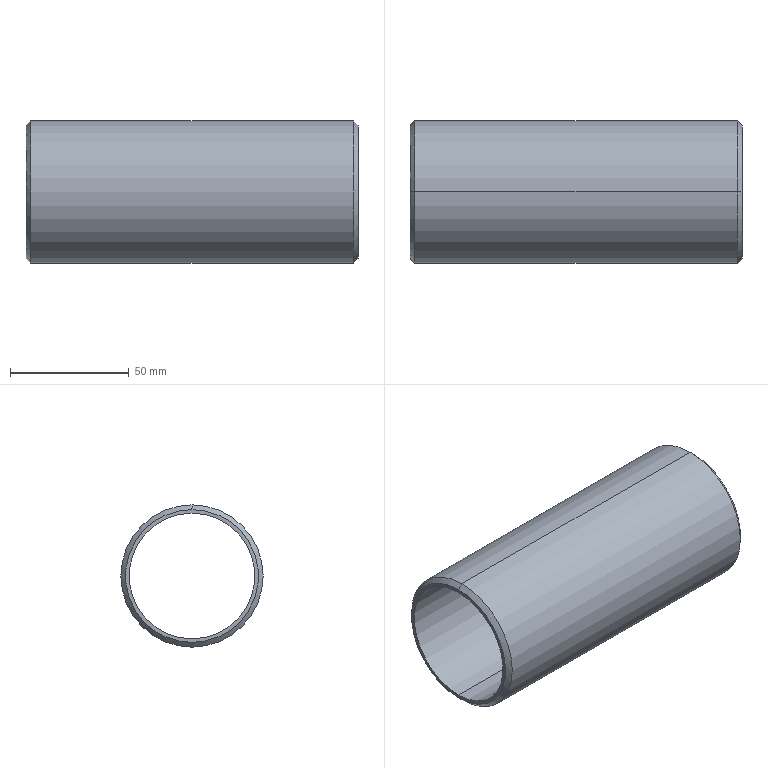Part | SolidWorks | features Chamfer 1, ExtruThin 1 | 1 solid | 10 faces | box 140 x 60 x 60 mm | volume 86238 mm3 | cone 4 | cylinder 4 | plane 2 | commonest cylinder face diameters 53 x2 60 x2
STEP:
#1=CARTESIAN_POINT('',(0.,0.,28.));
#2=VERTEX_POINT('',#1);
#3=CARTESIAN_POINT('',(0.,0.,-28.));
#4=VERTEX_POINT('',#3);
#5=CARTESIAN_POINT('',(0.,0.,0.));
#6=DIRECTION('',(-1.,0.,0.));
#7=DIRECTION('',(0.,0.,-1.));
#8=AXIS2_PLACEMENT_3D('',#5,#6,#7);
#9=CIRCLE('',#8,28.);
#10=EDGE_CURVE('',#2,#4,#9,.T.);
#11=ORIENTED_EDGE('',*,*,#10,.F.);
#12=CARTESIAN_POINT('',(2.,0.,30.));
#13=VERTEX_POINT('',#12);
#14=CARTESIAN_POINT('',(2.,0.,30.));
#15=DIRECTION('',(0.7071,0.,0.7071));
#16=VECTOR('',#15,1000.);
#17=LINE('',#14,#16);
#18=EDGE_CURVE('',#2,#13,#17,.T.);
#19=ORIENTED_EDGE('',*,*,#18,.T.);
#20=CARTESIAN_POINT('',(2.,0.,-30.));
#21=VERTEX_POINT('',#20);
#22=CARTESIAN_POINT('',(2.,0.,0.));
#23=DIRECTION('',(1.,0.,0.));
#24=DIRECTION('',(0.,0.,-1.));
#25=AXIS2_PLACEMENT_3D('',#22,#23,#24);
#26=CIRCLE('',#25,30.);
#27=EDGE_CURVE('',#21,#13,#26,.T.);
#28=ORIENTED_EDGE('',*,*,#27,.F.);
#29=CARTESIAN_POINT('',(2.,0.,-30.));
#30=DIRECTION('',(0.7071,0.,-0.7071));
#31=VECTOR('',#30,1000.);
#32=LINE('',#29,#31);
#33=EDGE_CURVE('',#4,#21,#32,.T.);
#34=ORIENTED_EDGE('',*,*,#33,.F.);
#35=EDGE_LOOP('',(#11,#19,#28,#34));
#36=FACE_OUTER_BOUND('',#35,.T.);
#37=CARTESIAN_POINT('',(2.,0.,0.));
#38=DIRECTION('',(1.,0.,0.));
#39=DIRECTION('',(0.,0.,-1.));
#40=AXIS2_PLACEMENT_3D('',#37,#38,#39);
#41=CONICAL_SURFACE('',#40,30.,0.7854);
#42=ADVANCED_FACE('',(#36),#41,.T.);
#43=CARTESIAN_POINT('',(140.,0.,-28.));
#44=VERTEX_POINT('',#43);
#45=CARTESIAN_POINT('',(140.,0.,28.));
#46=VERTEX_POINT('',#45);
#47=CARTESIAN_POINT('',(140.,0.,0.));
#48=DIRECTION('',(1.,0.,0.));
#49=DIRECTION('',(0.,0.,-1.));
#50=AXIS2_PLACEMENT_3D('',#47,#48,#49);
#51=CIRCLE('',#50,28.);
#52=EDGE_CURVE('',#44,#46,#51,.T.);
#53=ORIENTED_EDGE('',*,*,#52,.F.);
#54=CARTESIAN_POINT('',(138.,0.,-30.));
#55=VERTEX_POINT('',#54);
#56=CARTESIAN_POINT('',(140.,0.,-28.));
#57=DIRECTION('',(-0.7071,0.,-0.7071));
#58=VECTOR('',#57,1000.);
#59=LINE('',#56,#58);
#60=EDGE_CURVE('',#44,#55,#59,.T.);
#61=ORIENTED_EDGE('',*,*,#60,.T.);
#62=CARTESIAN_POINT('',(138.,0.,30.));
#63=VERTEX_POINT('',#62);
#64=CARTESIAN_POINT('',(138.,0.,0.));
#65=DIRECTION('',(-1.,0.,0.));
#66=DIRECTION('',(0.,0.,-1.));
#67=AXIS2_PLACEMENT_3D('',#64,#65,#66);
#68=CIRCLE('',#67,30.);
#69=EDGE_CURVE('',#63,#55,#68,.T.);
#70=ORIENTED_EDGE('',*,*,#69,.F.);
#71=CARTESIAN_POINT('',(140.,0.,28.));
#72=DIRECTION('',(-0.7071,0.,0.7071));
#73=VECTOR('',#72,1000.);
#74=LINE('',#71,#73);
#75=EDGE_CURVE('',#46,#63,#74,.T.);
#76=ORIENTED_EDGE('',*,*,#75,.F.);
#77=EDGE_LOOP('',(#53,#61,#70,#76));
#78=FACE_OUTER_BOUND('',#77,.T.);
#79=CARTESIAN_POINT('',(140.,0.,0.));
#80=DIRECTION('',(-1.,0.,0.));
#81=DIRECTION('',(0.,0.,1.));
#82=AXIS2_PLACEMENT_3D('',#79,#80,#81);
#83=CONICAL_SURFACE('',#82,28.,0.7854);
#84=ADVANCED_FACE('',(#78),#83,.T.);
#85=CARTESIAN_POINT('',(140.,0.,26.5));
#86=VERTEX_POINT('',#85);
#87=CARTESIAN_POINT('',(140.,0.,-26.5));
#88=VERTEX_POINT('',#87);
#89=CARTESIAN_POINT('',(140.,0.,0.));
#90=DIRECTION('',(1.,0.,0.));
#91=DIRECTION('',(0.,0.,-1.));
#92=AXIS2_PLACEMENT_3D('',#89,#90,#91);
#93=CIRCLE('',#92,26.5);
#94=EDGE_CURVE('',#86,#88,#93,.T.);
#95=ORIENTED_EDGE('',*,*,#94,.T.);
#96=CARTESIAN_POINT('',(0.,0.,-26.5));
#97=VERTEX_POINT('',#96);
#98=CARTESIAN_POINT('',(140.,0.,-26.5));
#99=DIRECTION('',(-1.,0.,0.));
#100=VECTOR('',#99,1000.);
#101=LINE('',#98,#100);
#102=EDGE_CURVE('',#88,#97,#101,.T.);
#103=ORIENTED_EDGE('',*,*,#102,.T.);
#104=CARTESIAN_POINT('',(0.,0.,26.5));
#105=VERTEX_POINT('',#104);
#106=CARTESIAN_POINT('',(0.,0.,0.));
#107=DIRECTION('',(1.,0.,0.));
#108=DIRECTION('',(0.,0.,-1.));
#109=AXIS2_PLACEMENT_3D('',#106,#107,#108);
#110=CIRCLE('',#109,26.5);
#111=EDGE_CURVE('',#105,#97,#110,.T.);
#112=ORIENTED_EDGE('',*,*,#111,.F.);
#113=CARTESIAN_POINT('',(140.,0.,26.5));
#114=DIRECTION('',(-1.,0.,0.));
#115=VECTOR('',#114,1000.);
#116=LINE('',#113,#115);
#117=EDGE_CURVE('',#86,#105,#116,.T.);
#118=ORIENTED_EDGE('',*,*,#117,.F.);
#119=EDGE_LOOP('',(#95,#103,#112,#118));
#120=FACE_OUTER_BOUND('',#119,.T.);
#121=CARTESIAN_POINT('',(140.,0.,0.));
#122=DIRECTION('',(-1.,0.,0.));
#123=DIRECTION('',(0.,0.,1.));
#124=AXIS2_PLACEMENT_3D('',#121,#122,#123);
#125=CYLINDRICAL_SURFACE('',#124,26.5);
#126=ADVANCED_FACE('',(#120),#125,.F.);
#127=ORIENTED_EDGE('',*,*,#69,.T.);
#128=CARTESIAN_POINT('',(140.,0.,-30.));
#129=DIRECTION('',(-1.,0.,0.));
#130=VECTOR('',#129,1000.);
#131=LINE('',#128,#130);
#132=EDGE_CURVE('',#55,#21,#131,.T.);
#133=ORIENTED_EDGE('',*,*,#132,.T.);
#134=ORIENTED_EDGE('',*,*,#27,.T.);
#135=CARTESIAN_POINT('',(140.,0.,30.));
#136=DIRECTION('',(-1.,0.,0.));
#137=VECTOR('',#136,1000.);
#138=LINE('',#135,#137);
#139=EDGE_CURVE('',#63,#13,#138,.T.);
#140=ORIENTED_EDGE('',*,*,#139,.F.);
#141=EDGE_LOOP('',(#127,#133,#134,#140));
#142=FACE_OUTER_BOUND('',#141,.T.);
#143=CARTESIAN_POINT('',(140.,0.,0.));
#144=DIRECTION('',(-1.,0.,0.));
#145=DIRECTION('',(0.,0.,1.));
#146=AXIS2_PLACEMENT_3D('',#143,#144,#145);
#147=CYLINDRICAL_SURFACE('',#146,30.);
#148=ADVANCED_FACE('',(#142),#147,.T.);
#149=CARTESIAN_POINT('',(140.,0.,0.));
#150=DIRECTION('',(1.,0.,0.));
#151=DIRECTION('',(0.,0.,-1.));
#152=AXIS2_PLACEMENT_3D('',#149,#150,#151);
#153=CIRCLE('',#152,28.);
#154=EDGE_CURVE('',#46,#44,#153,.T.);
#155=ORIENTED_EDGE('',*,*,#154,.T.);
#156=ORIENTED_EDGE('',*,*,#52,.T.);
#157=EDGE_LOOP('',(#155,#156));
#158=FACE_OUTER_BOUND('',#157,.T.);
#159=ORIENTED_EDGE('',*,*,#94,.F.);
#160=CARTESIAN_POINT('',(140.,0.,0.));
#161=DIRECTION('',(1.,0.,0.));
#162=DIRECTION('',(0.,0.,-1.));
#163=AXIS2_PLACEMENT_3D('',#160,#161,#162);
#164=CIRCLE('',#163,26.5);
#165=EDGE_CURVE('',#88,#86,#164,.T.);
#166=ORIENTED_EDGE('',*,*,#165,.F.);
#167=EDGE_LOOP('',(#159,#166));
#168=FACE_BOUND('',#167,.T.);
#169=CARTESIAN_POINT('',(140.,0.,0.));
#170=DIRECTION('',(1.,0.,0.));
#171=DIRECTION('',(0.,0.,-1.));
#172=AXIS2_PLACEMENT_3D('',#169,#170,#171);
#173=PLANE('',#172);
#174=ADVANCED_FACE('',(#158,#168),#173,.T.);
#175=CARTESIAN_POINT('',(0.,0.,0.));
#176=DIRECTION('',(-1.,0.,0.));
#177=DIRECTION('',(0.,0.,-1.));
#178=AXIS2_PLACEMENT_3D('',#175,#176,#177);
#179=CIRCLE('',#178,28.);
#180=EDGE_CURVE('',#4,#2,#179,.T.);
#181=ORIENTED_EDGE('',*,*,#180,.T.);
#182=ORIENTED_EDGE('',*,*,#10,.T.);
#183=EDGE_LOOP('',(#181,#182));
#184=FACE_OUTER_BOUND('',#183,.T.);
#185=ORIENTED_EDGE('',*,*,#111,.T.);
#186=CARTESIAN_POINT('',(0.,0.,0.));
#187=DIRECTION('',(1.,0.,0.));
#188=DIRECTION('',(0.,0.,-1.));
#189=AXIS2_PLACEMENT_3D('',#186,#187,#188);
#190=CIRCLE('',#189,26.5);
#191=EDGE_CURVE('',#97,#105,#190,.T.);
#192=ORIENTED_EDGE('',*,*,#191,.T.);
#193=EDGE_LOOP('',(#185,#192));
#194=FACE_BOUND('',#193,.T.);
#195=CARTESIAN_POINT('',(0.,0.,0.));
#196=DIRECTION('',(1.,0.,0.));
#197=DIRECTION('',(0.,0.,-1.));
#198=AXIS2_PLACEMENT_3D('',#195,#196,#197);
#199=PLANE('',#198);
#200=ADVANCED_FACE('',(#184,#194),#199,.F.);
#201=ORIENTED_EDGE('',*,*,#132,.F.);
#202=CARTESIAN_POINT('',(138.,0.,0.));
#203=DIRECTION('',(-1.,0.,0.));
#204=DIRECTION('',(0.,0.,-1.));
#205=AXIS2_PLACEMENT_3D('',#202,#203,#204);
#206=CIRCLE('',#205,30.);
#207=EDGE_CURVE('',#55,#63,#206,.T.);
#208=ORIENTED_EDGE('',*,*,#207,.T.);
#209=ORIENTED_EDGE('',*,*,#139,.T.);
#210=CARTESIAN_POINT('',(2.,0.,0.));
#211=DIRECTION('',(1.,0.,0.));
#212=DIRECTION('',(0.,0.,-1.));
#213=AXIS2_PLACEMENT_3D('',#210,#211,#212);
#214=CIRCLE('',#213,30.);
#215=EDGE_CURVE('',#13,#21,#214,.T.);
#216=ORIENTED_EDGE('',*,*,#215,.T.);
#217=EDGE_LOOP('',(#201,#208,#209,#216));
#218=FACE_OUTER_BOUND('',#217,.T.);
#219=CARTESIAN_POINT('',(140.,0.,0.));
#220=DIRECTION('',(-1.,0.,0.));
#221=DIRECTION('',(0.,0.,1.));
#222=AXIS2_PLACEMENT_3D('',#219,#220,#221);
#223=CYLINDRICAL_SURFACE('',#222,30.);
#224=ADVANCED_FACE('',(#218),#223,.T.);
#225=ORIENTED_EDGE('',*,*,#102,.F.);
#226=ORIENTED_EDGE('',*,*,#165,.T.);
#227=ORIENTED_EDGE('',*,*,#117,.T.);
#228=ORIENTED_EDGE('',*,*,#191,.F.);
#229=EDGE_LOOP('',(#225,#226,#227,#228));
#230=FACE_OUTER_BOUND('',#229,.T.);
#231=CARTESIAN_POINT('',(140.,0.,0.));
#232=DIRECTION('',(-1.,0.,0.));
#233=DIRECTION('',(0.,0.,1.));
#234=AXIS2_PLACEMENT_3D('',#231,#232,#233);
#235=CYLINDRICAL_SURFACE('',#234,26.5);
#236=ADVANCED_FACE('',(#230),#235,.F.);
#237=ORIENTED_EDGE('',*,*,#60,.F.);
#238=ORIENTED_EDGE('',*,*,#154,.F.);
#239=ORIENTED_EDGE('',*,*,#75,.T.);
#240=ORIENTED_EDGE('',*,*,#207,.F.);
#241=EDGE_LOOP('',(#237,#238,#239,#240));
#242=FACE_OUTER_BOUND('',#241,.T.);
#243=CARTESIAN_POINT('',(140.,0.,0.));
#244=DIRECTION('',(-1.,0.,0.));
#245=DIRECTION('',(0.,0.,1.));
#246=AXIS2_PLACEMENT_3D('',#243,#244,#245);
#247=CONICAL_SURFACE('',#246,28.,0.7854);
#248=ADVANCED_FACE('',(#242),#247,.T.);
#249=ORIENTED_EDGE('',*,*,#18,.F.);
#250=ORIENTED_EDGE('',*,*,#180,.F.);
#251=ORIENTED_EDGE('',*,*,#33,.T.);
#252=ORIENTED_EDGE('',*,*,#215,.F.);
#253=EDGE_LOOP('',(#249,#250,#251,#252));
#254=FACE_OUTER_BOUND('',#253,.T.);
#255=CARTESIAN_POINT('',(2.,0.,0.));
#256=DIRECTION('',(1.,0.,0.));
#257=DIRECTION('',(0.,0.,-1.));
#258=AXIS2_PLACEMENT_3D('',#255,#256,#257);
#259=CONICAL_SURFACE('',#258,30.,0.7854);
#260=ADVANCED_FACE('',(#254),#259,.T.);
#261=CLOSED_SHELL('',(#42,#84,#126,#148,#174,#200,#224,#236,#248,#260));
#262=MANIFOLD_SOLID_BREP('',#261);
#263=CARTESIAN_POINT('',(0.,0.,0.));
#264=DIRECTION('',(0.,0.,1.));
#265=DIRECTION('',(1.,0.,0.));
#266=AXIS2_PLACEMENT_3D('',#263,#264,#265);
#267=(LENGTH_UNIT()NAMED_UNIT(*)SI_UNIT(.MILLI.,.METRE.));
#268=UNCERTAINTY_MEASURE_WITH_UNIT(LENGTH_MEASURE(0.00001),#267,'','');
#269=(NAMED_UNIT(*)PLANE_ANGLE_UNIT()SI_UNIT($,.RADIAN.));
#270=(NAMED_UNIT(*)SI_UNIT($,.STERADIAN.)SOLID_ANGLE_UNIT());
#271=(GEOMETRIC_REPRESENTATION_CONTEXT(3)GLOBAL_UNCERTAINTY_ASSIGNED_CONTEXT((#268))GLOBAL_UNIT_ASSIGNED_CONTEXT((#267,#269,#270))REPRESENTATION_CONTEXT('',''));
#272=ADVANCED_BREP_SHAPE_REPRESENTATION('',(#262,#266),#271);